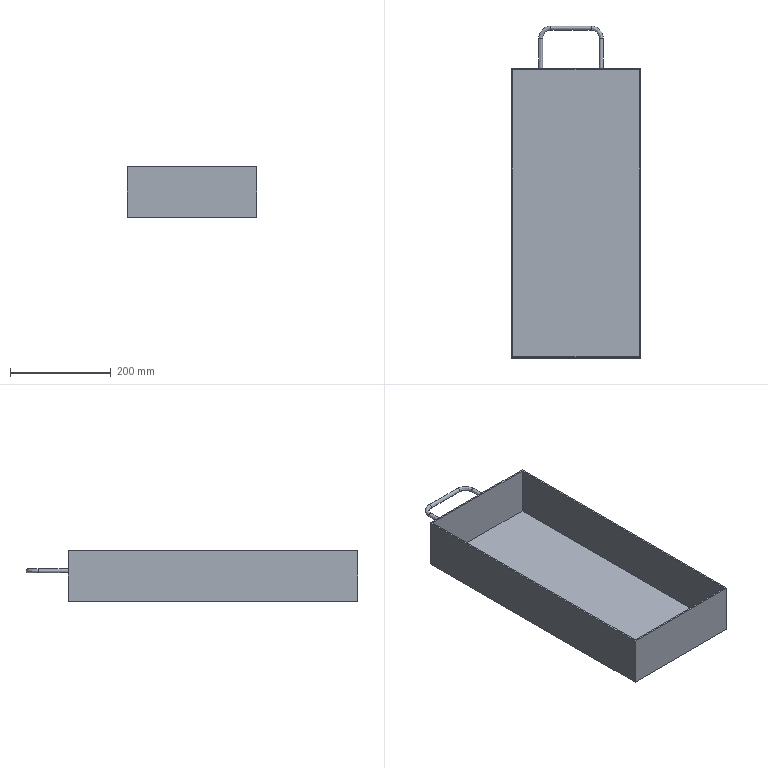Part | NX | features solid 2 | 1 solid | 16 faces | box 258 x 659 x 100 mm | volume 939581 mm3 | plane 11 | spline 5